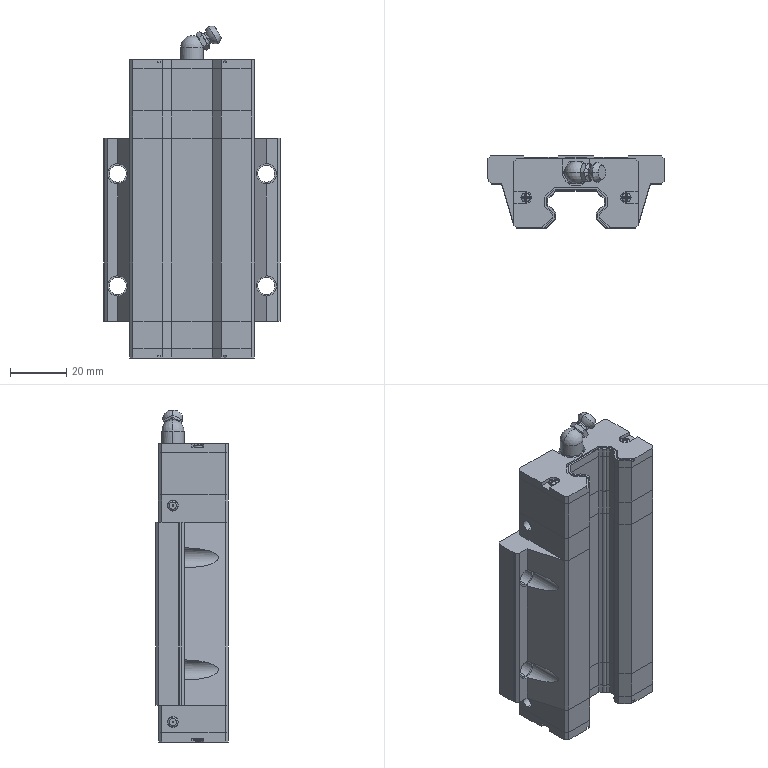Part | SolidWorks | features ICE 22, Extrusion 5, MirrorPattern 5, Fillet 4, MirrorSolid 4, Chamfer 3, RevCut 3, Dome 2, LPattern 2, Revolution 2, DeleteBody 1, LibraryFeature 1 | 7 solids | 481 faces | box 63 x 25.7 x 118.4 mm | volume 108820 mm3 | plane 331 | cylinder 92 | torus 25 | cone 23 | sphere 10 | commonest cylinder face diameters 1.817 x36 3.93 x12 0.531 x8 3.352 x8 6 x8 7.2 x8